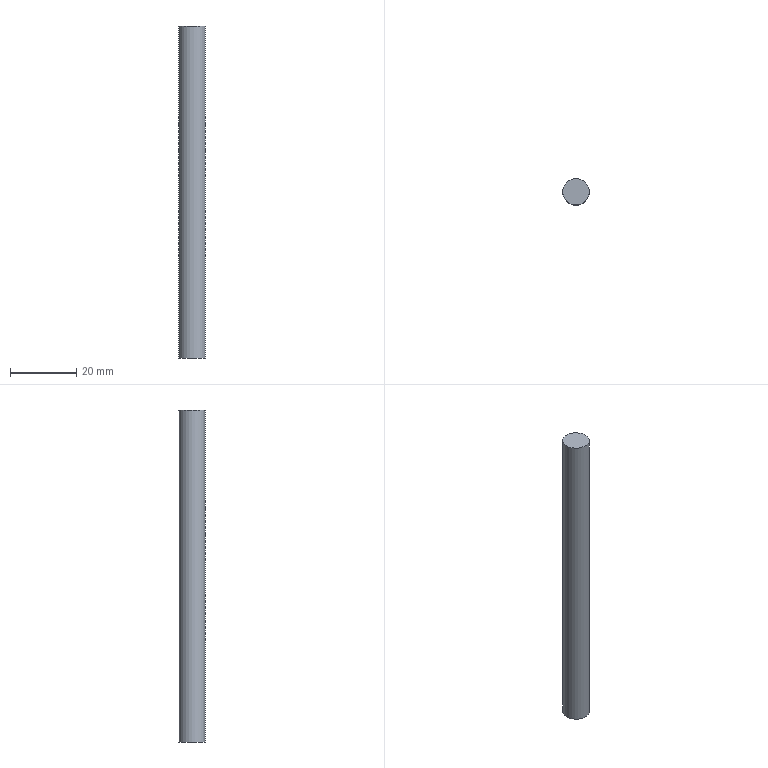Part | NX | features BREP 1, DATUM_CSYS 1 | 1 solid | 3 faces | box 8 x 8 x 100 mm | volume 5027 mm3 | plane 2 | cylinder 1 | commonest cylinder face diameters 8 x1
STEP:
#1=CARTESIAN_POINT('',(4.,0.,0.));
#2=VERTEX_POINT('',#1);
#3=CARTESIAN_POINT('',(0.,0.,0.));
#4=DIRECTION('',(0.,0.,1.));
#5=DIRECTION('',(1.,0.,0.));
#6=AXIS2_PLACEMENT_3D('',#3,#4,#5);
#7=CIRCLE('',#6,4.);
#8=EDGE_CURVE('',#2,#2,#7,.T.);
#9=ORIENTED_EDGE('',*,*,#8,.F.);
#10=EDGE_LOOP('',(#9));
#11=FACE_BOUND('',#10,.T.);
#12=CARTESIAN_POINT('',(0.,0.,0.));
#13=DIRECTION('',(0.,0.,1.));
#14=DIRECTION('',(-1.,0.,0.));
#15=AXIS2_PLACEMENT_3D('',#12,#13,#14);
#16=PLANE('',#15);
#17=ADVANCED_FACE('',(#11),#16,.F.);
#18=CARTESIAN_POINT('',(4.,0.,100.));
#19=VERTEX_POINT('',#18);
#20=CARTESIAN_POINT('',(0.,0.,100.));
#21=DIRECTION('',(0.,0.,1.));
#22=DIRECTION('',(1.,0.,0.));
#23=AXIS2_PLACEMENT_3D('',#20,#21,#22);
#24=CIRCLE('',#23,4.);
#25=EDGE_CURVE('',#19,#19,#24,.T.);
#26=ORIENTED_EDGE('',*,*,#25,.T.);
#27=EDGE_LOOP('',(#26));
#28=FACE_BOUND('',#27,.T.);
#29=CARTESIAN_POINT('',(0.,0.,100.));
#30=DIRECTION('',(0.,0.,1.));
#31=DIRECTION('',(-1.,0.,0.));
#32=AXIS2_PLACEMENT_3D('',#29,#30,#31);
#33=PLANE('',#32);
#34=ADVANCED_FACE('',(#28),#33,.T.);
#35=ORIENTED_EDGE('',*,*,#8,.T.);
#36=CARTESIAN_POINT('',(4.,0.,0.));
#37=DIRECTION('',(0.,0.,1.));
#38=VECTOR('',#37,1000.);
#39=LINE('',#36,#38);
#40=EDGE_CURVE('',#2,#19,#39,.T.);
#41=ORIENTED_EDGE('',*,*,#40,.T.);
#42=ORIENTED_EDGE('',*,*,#25,.F.);
#43=ORIENTED_EDGE('',*,*,#40,.F.);
#44=EDGE_LOOP('',(#35,#41,#42,#43));
#45=FACE_BOUND('',#44,.T.);
#46=CARTESIAN_POINT('',(0.,0.,0.));
#47=DIRECTION('',(0.,0.,1.));
#48=DIRECTION('',(-1.,0.,0.));
#49=AXIS2_PLACEMENT_3D('',#46,#47,#48);
#50=CYLINDRICAL_SURFACE('',#49,4.);
#51=ADVANCED_FACE('',(#45),#50,.T.);
#52=CLOSED_SHELL('',(#17,#34,#51));
#53=MANIFOLD_SOLID_BREP('',#52);
#54=(LENGTH_UNIT()NAMED_UNIT(*)SI_UNIT(.MILLI.,.METRE.));
#55=UNCERTAINTY_MEASURE_WITH_UNIT(LENGTH_MEASURE(0.00001),#54,'','');
#56=(NAMED_UNIT(*)PLANE_ANGLE_UNIT()SI_UNIT($,.RADIAN.));
#57=(NAMED_UNIT(*)SI_UNIT($,.STERADIAN.)SOLID_ANGLE_UNIT());
#58=(GEOMETRIC_REPRESENTATION_CONTEXT(3)GLOBAL_UNCERTAINTY_ASSIGNED_CONTEXT((#55))GLOBAL_UNIT_ASSIGNED_CONTEXT((#54,#56,#57))REPRESENTATION_CONTEXT('',''));
#59=ADVANCED_BREP_SHAPE_REPRESENTATION('',(#53),#58);